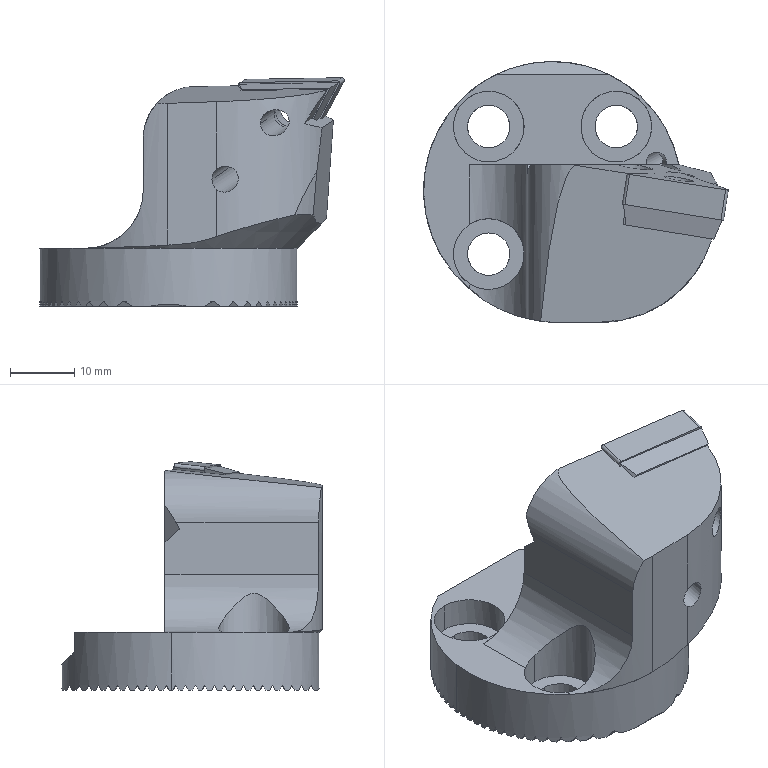Part | 3 solids | 231 faces | volume 22263 mm3 | plane 184 | cylinder 43 | cone 4 | commonest cylinder face diameters 6.6 x6 11 x6 4 x5 4.5 x4 0.8 x3 1.5 x2